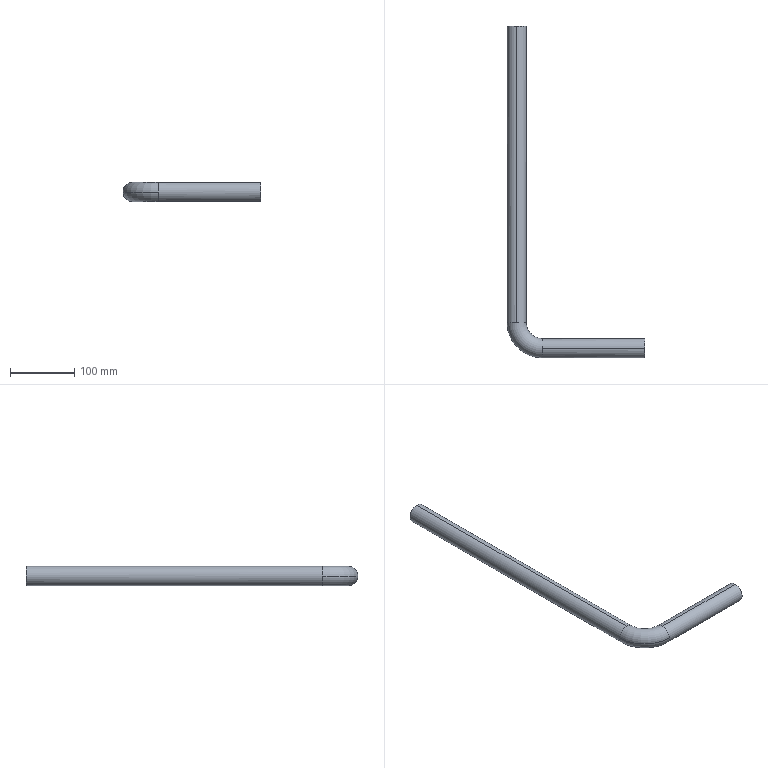Part | SolidWorks | features Sweep 1 | 1 solid | 14 faces | box 215 x 517 x 30 mm | volume 120482 mm3 | cylinder 8 | torus 4 | plane 2 | commonest cylinder face diameters 26 x4 30 x4
STEP:
#1=CARTESIAN_POINT('',(40.,0.,13.));
#2=VERTEX_POINT('',#1);
#3=CARTESIAN_POINT('',(40.,-13.,0.));
#4=VERTEX_POINT('',#3);
#5=CARTESIAN_POINT('',(40.,0.,0.));
#6=DIRECTION('',(1.,0.,0.));
#7=DIRECTION('',(0.,0.,1.));
#8=AXIS2_PLACEMENT_3D('',#5,#6,#7);
#9=CIRCLE('',#8,13.);
#10=EDGE_CURVE('',#2,#4,#9,.T.);
#11=ORIENTED_EDGE('',*,*,#10,.T.);
#12=CARTESIAN_POINT('',(-13.,40.,0.));
#13=VERTEX_POINT('',#12);
#14=CARTESIAN_POINT('',(40.,40.,0.));
#15=DIRECTION('',(0.,0.,-1.));
#16=DIRECTION('',(-1.,0.,0.));
#17=AXIS2_PLACEMENT_3D('',#14,#15,#16);
#18=CIRCLE('',#17,53.);
#19=EDGE_CURVE('',#4,#13,#18,.T.);
#20=ORIENTED_EDGE('',*,*,#19,.T.);
#21=CARTESIAN_POINT('',(0.,40.,13.));
#22=VERTEX_POINT('',#21);
#23=CARTESIAN_POINT('',(0.,40.,0.));
#24=DIRECTION('',(0.,-1.,0.));
#25=DIRECTION('',(0.,0.,-1.));
#26=AXIS2_PLACEMENT_3D('',#23,#24,#25);
#27=CIRCLE('',#26,13.);
#28=EDGE_CURVE('',#22,#13,#27,.T.);
#29=ORIENTED_EDGE('',*,*,#28,.F.);
#30=CARTESIAN_POINT('',(13.,40.,0.));
#31=VERTEX_POINT('',#30);
#32=CARTESIAN_POINT('',(0.,40.,0.));
#33=DIRECTION('',(0.,-1.,0.));
#34=DIRECTION('',(0.,0.,-1.));
#35=AXIS2_PLACEMENT_3D('',#32,#33,#34);
#36=CIRCLE('',#35,13.);
#37=EDGE_CURVE('',#31,#22,#36,.T.);
#38=ORIENTED_EDGE('',*,*,#37,.F.);
#39=CARTESIAN_POINT('',(40.,13.,0.));
#40=VERTEX_POINT('',#39);
#41=CARTESIAN_POINT('',(40.,40.,0.));
#42=DIRECTION('',(0.,0.,-1.));
#43=DIRECTION('',(-1.,0.,0.));
#44=AXIS2_PLACEMENT_3D('',#41,#42,#43);
#45=CIRCLE('',#44,27.);
#46=EDGE_CURVE('',#40,#31,#45,.T.);
#47=ORIENTED_EDGE('',*,*,#46,.F.);
#48=CARTESIAN_POINT('',(40.,0.,0.));
#49=DIRECTION('',(1.,0.,0.));
#50=DIRECTION('',(0.,0.,1.));
#51=AXIS2_PLACEMENT_3D('',#48,#49,#50);
#52=CIRCLE('',#51,13.);
#53=EDGE_CURVE('',#40,#2,#52,.T.);
#54=ORIENTED_EDGE('',*,*,#53,.T.);
#55=EDGE_LOOP('',(#11,#20,#29,#38,#47,#54));
#56=FACE_OUTER_BOUND('',#55,.T.);
#57=CARTESIAN_POINT('',(40.,40.,0.));
#58=DIRECTION('',(0.,0.,-1.));
#59=DIRECTION('',(-1.,0.,0.));
#60=AXIS2_PLACEMENT_3D('',#57,#58,#59);
#61=TOROIDAL_SURFACE('',#60,40.,13.);
#62=ADVANCED_FACE('',(#56),#61,.F.);
#63=CARTESIAN_POINT('',(40.,-15.,0.));
#64=VERTEX_POINT('',#63);
#65=CARTESIAN_POINT('',(40.,0.,-15.));
#66=VERTEX_POINT('',#65);
#67=CARTESIAN_POINT('',(40.,0.,0.));
#68=DIRECTION('',(1.,0.,0.));
#69=DIRECTION('',(0.,0.,-1.));
#70=AXIS2_PLACEMENT_3D('',#67,#68,#69);
#71=CIRCLE('',#70,15.);
#72=EDGE_CURVE('',#64,#66,#71,.T.);
#73=ORIENTED_EDGE('',*,*,#72,.F.);
#74=CARTESIAN_POINT('',(-15.,40.,0.));
#75=VERTEX_POINT('',#74);
#76=CARTESIAN_POINT('',(40.,40.,0.));
#77=DIRECTION('',(0.,0.,-1.));
#78=DIRECTION('',(-1.,0.,0.));
#79=AXIS2_PLACEMENT_3D('',#76,#77,#78);
#80=CIRCLE('',#79,55.);
#81=EDGE_CURVE('',#64,#75,#80,.T.);
#82=ORIENTED_EDGE('',*,*,#81,.T.);
#83=CARTESIAN_POINT('',(0.,40.,-15.));
#84=VERTEX_POINT('',#83);
#85=CARTESIAN_POINT('',(0.,40.,0.));
#86=DIRECTION('',(0.,-1.,0.));
#87=DIRECTION('',(0.,0.,-1.));
#88=AXIS2_PLACEMENT_3D('',#85,#86,#87);
#89=CIRCLE('',#88,15.);
#90=EDGE_CURVE('',#75,#84,#89,.T.);
#91=ORIENTED_EDGE('',*,*,#90,.T.);
#92=CARTESIAN_POINT('',(15.,40.,0.));
#93=VERTEX_POINT('',#92);
#94=CARTESIAN_POINT('',(0.,40.,0.));
#95=DIRECTION('',(0.,-1.,0.));
#96=DIRECTION('',(0.,0.,-1.));
#97=AXIS2_PLACEMENT_3D('',#94,#95,#96);
#98=CIRCLE('',#97,15.);
#99=EDGE_CURVE('',#84,#93,#98,.T.);
#100=ORIENTED_EDGE('',*,*,#99,.T.);
#101=CARTESIAN_POINT('',(40.,15.,0.));
#102=VERTEX_POINT('',#101);
#103=CARTESIAN_POINT('',(40.,40.,0.));
#104=DIRECTION('',(0.,0.,-1.));
#105=DIRECTION('',(-1.,0.,0.));
#106=AXIS2_PLACEMENT_3D('',#103,#104,#105);
#107=CIRCLE('',#106,25.);
#108=EDGE_CURVE('',#102,#93,#107,.T.);
#109=ORIENTED_EDGE('',*,*,#108,.F.);
#110=CARTESIAN_POINT('',(40.,0.,0.));
#111=DIRECTION('',(1.,0.,0.));
#112=DIRECTION('',(0.,0.,-1.));
#113=AXIS2_PLACEMENT_3D('',#110,#111,#112);
#114=CIRCLE('',#113,15.);
#115=EDGE_CURVE('',#66,#102,#114,.T.);
#116=ORIENTED_EDGE('',*,*,#115,.F.);
#117=EDGE_LOOP('',(#73,#82,#91,#100,#109,#116));
#118=FACE_OUTER_BOUND('',#117,.T.);
#119=CARTESIAN_POINT('',(40.,40.,0.));
#120=DIRECTION('',(0.,0.,-1.));
#121=DIRECTION('',(-1.,0.,0.));
#122=AXIS2_PLACEMENT_3D('',#119,#120,#121);
#123=TOROIDAL_SURFACE('',#122,40.,15.);
#124=ADVANCED_FACE('',(#118),#123,.T.);
#125=ORIENTED_EDGE('',*,*,#28,.T.);
#126=CARTESIAN_POINT('',(0.,40.,-13.));
#127=VERTEX_POINT('',#126);
#128=CARTESIAN_POINT('',(0.,40.,0.));
#129=DIRECTION('',(0.,-1.,0.));
#130=DIRECTION('',(0.,0.,-1.));
#131=AXIS2_PLACEMENT_3D('',#128,#129,#130);
#132=CIRCLE('',#131,13.);
#133=EDGE_CURVE('',#13,#127,#132,.T.);
#134=ORIENTED_EDGE('',*,*,#133,.T.);
#135=CARTESIAN_POINT('',(0.,502.,-13.));
#136=VERTEX_POINT('',#135);
#137=CARTESIAN_POINT('',(0.,40.,-13.));
#138=DIRECTION('',(0.,1.,0.));
#139=VECTOR('',#138,1000.);
#140=LINE('',#137,#139);
#141=EDGE_CURVE('',#127,#136,#140,.T.);
#142=ORIENTED_EDGE('',*,*,#141,.T.);
#143=CARTESIAN_POINT('',(0.,502.,13.));
#144=VERTEX_POINT('',#143);
#145=CARTESIAN_POINT('',(0.,502.,0.));
#146=DIRECTION('',(0.,-1.,0.));
#147=DIRECTION('',(0.,0.,-1.));
#148=AXIS2_PLACEMENT_3D('',#145,#146,#147);
#149=CIRCLE('',#148,13.);
#150=EDGE_CURVE('',#144,#136,#149,.T.);
#151=ORIENTED_EDGE('',*,*,#150,.F.);
#152=CARTESIAN_POINT('',(0.,40.,13.));
#153=DIRECTION('',(0.,1.,0.));
#154=VECTOR('',#153,1000.);
#155=LINE('',#152,#154);
#156=EDGE_CURVE('',#22,#144,#155,.T.);
#157=ORIENTED_EDGE('',*,*,#156,.F.);
#158=EDGE_LOOP('',(#125,#134,#142,#151,#157));
#159=FACE_OUTER_BOUND('',#158,.T.);
#160=CARTESIAN_POINT('',(0.,40.,0.));
#161=DIRECTION('',(0.,1.,0.));
#162=DIRECTION('',(0.,0.,1.));
#163=AXIS2_PLACEMENT_3D('',#160,#161,#162);
#164=CYLINDRICAL_SURFACE('',#163,13.);
#165=ADVANCED_FACE('',(#159),#164,.F.);
#166=CARTESIAN_POINT('',(200.,0.,13.));
#167=VERTEX_POINT('',#166);
#168=CARTESIAN_POINT('',(200.,0.,-13.));
#169=VERTEX_POINT('',#168);
#170=CARTESIAN_POINT('',(200.,0.,0.));
#171=DIRECTION('',(1.,0.,0.));
#172=DIRECTION('',(0.,0.,-1.));
#173=AXIS2_PLACEMENT_3D('',#170,#171,#172);
#174=CIRCLE('',#173,13.);
#175=EDGE_CURVE('',#167,#169,#174,.T.);
#176=ORIENTED_EDGE('',*,*,#175,.T.);
#177=CARTESIAN_POINT('',(40.,0.,-13.));
#178=VERTEX_POINT('',#177);
#179=CARTESIAN_POINT('',(200.,0.,-13.));
#180=DIRECTION('',(-1.,0.,0.));
#181=VECTOR('',#180,1000.);
#182=LINE('',#179,#181);
#183=EDGE_CURVE('',#169,#178,#182,.T.);
#184=ORIENTED_EDGE('',*,*,#183,.T.);
#185=CARTESIAN_POINT('',(40.,0.,0.));
#186=DIRECTION('',(1.,0.,0.));
#187=DIRECTION('',(0.,0.,1.));
#188=AXIS2_PLACEMENT_3D('',#185,#186,#187);
#189=CIRCLE('',#188,13.);
#190=EDGE_CURVE('',#4,#178,#189,.T.);
#191=ORIENTED_EDGE('',*,*,#190,.F.);
#192=ORIENTED_EDGE('',*,*,#10,.F.);
#193=CARTESIAN_POINT('',(200.,0.,13.));
#194=DIRECTION('',(-1.,0.,0.));
#195=VECTOR('',#194,1000.);
#196=LINE('',#193,#195);
#197=EDGE_CURVE('',#167,#2,#196,.T.);
#198=ORIENTED_EDGE('',*,*,#197,.F.);
#199=EDGE_LOOP('',(#176,#184,#191,#192,#198));
#200=FACE_OUTER_BOUND('',#199,.T.);
#201=CARTESIAN_POINT('',(200.,0.,0.));
#202=DIRECTION('',(-1.,0.,0.));
#203=DIRECTION('',(0.,0.,1.));
#204=AXIS2_PLACEMENT_3D('',#201,#202,#203);
#205=CYLINDRICAL_SURFACE('',#204,13.);
#206=ADVANCED_FACE('',(#200),#205,.F.);
#207=ORIENTED_EDGE('',*,*,#99,.F.);
#208=CARTESIAN_POINT('',(0.,502.,-15.));
#209=VERTEX_POINT('',#208);
#210=CARTESIAN_POINT('',(0.,40.,-15.));
#211=DIRECTION('',(0.,1.,0.));
#212=VECTOR('',#211,1000.);
#213=LINE('',#210,#212);
#214=EDGE_CURVE('',#84,#209,#213,.T.);
#215=ORIENTED_EDGE('',*,*,#214,.T.);
#216=CARTESIAN_POINT('',(0.,502.,15.));
#217=VERTEX_POINT('',#216);
#218=CARTESIAN_POINT('',(0.,502.,0.));
#219=DIRECTION('',(0.,-1.,0.));
#220=DIRECTION('',(0.,0.,-1.));
#221=AXIS2_PLACEMENT_3D('',#218,#219,#220);
#222=CIRCLE('',#221,15.);
#223=EDGE_CURVE('',#209,#217,#222,.T.);
#224=ORIENTED_EDGE('',*,*,#223,.T.);
#225=CARTESIAN_POINT('',(0.,40.,15.));
#226=VERTEX_POINT('',#225);
#227=CARTESIAN_POINT('',(0.,40.,15.));
#228=DIRECTION('',(0.,1.,0.));
#229=VECTOR('',#228,1000.);
#230=LINE('',#227,#229);
#231=EDGE_CURVE('',#226,#217,#230,.T.);
#232=ORIENTED_EDGE('',*,*,#231,.F.);
#233=CARTESIAN_POINT('',(0.,40.,0.));
#234=DIRECTION('',(0.,-1.,0.));
#235=DIRECTION('',(0.,0.,-1.));
#236=AXIS2_PLACEMENT_3D('',#233,#234,#235);
#237=CIRCLE('',#236,15.);
#238=EDGE_CURVE('',#93,#226,#237,.T.);
#239=ORIENTED_EDGE('',*,*,#238,.F.);
#240=EDGE_LOOP('',(#207,#215,#224,#232,#239));
#241=FACE_OUTER_BOUND('',#240,.T.);
#242=CARTESIAN_POINT('',(0.,40.,0.));
#243=DIRECTION('',(0.,1.,0.));
#244=DIRECTION('',(0.,0.,1.));
#245=AXIS2_PLACEMENT_3D('',#242,#243,#244);
#246=CYLINDRICAL_SURFACE('',#245,15.);
#247=ADVANCED_FACE('',(#241),#246,.T.);
#248=CARTESIAN_POINT('',(200.,0.,-15.));
#249=VERTEX_POINT('',#248);
#250=CARTESIAN_POINT('',(200.,0.,15.));
#251=VERTEX_POINT('',#250);
#252=CARTESIAN_POINT('',(200.,0.,0.));
#253=DIRECTION('',(1.,0.,0.));
#254=DIRECTION('',(0.,0.,-1.));
#255=AXIS2_PLACEMENT_3D('',#252,#253,#254);
#256=CIRCLE('',#255,15.);
#257=EDGE_CURVE('',#249,#251,#256,.T.);
#258=ORIENTED_EDGE('',*,*,#257,.F.);
#259=CARTESIAN_POINT('',(200.,0.,-15.));
#260=DIRECTION('',(-1.,0.,0.));
#261=VECTOR('',#260,1000.);
#262=LINE('',#259,#261);
#263=EDGE_CURVE('',#249,#66,#262,.T.);
#264=ORIENTED_EDGE('',*,*,#263,.T.);
#265=ORIENTED_EDGE('',*,*,#115,.T.);
#266=CARTESIAN_POINT('',(40.,0.,15.));
#267=VERTEX_POINT('',#266);
#268=CARTESIAN_POINT('',(40.,0.,0.));
#269=DIRECTION('',(1.,0.,0.));
#270=DIRECTION('',(0.,0.,-1.));
#271=AXIS2_PLACEMENT_3D('',#268,#269,#270);
#272=CIRCLE('',#271,15.);
#273=EDGE_CURVE('',#102,#267,#272,.T.);
#274=ORIENTED_EDGE('',*,*,#273,.T.);
#275=CARTESIAN_POINT('',(200.,0.,15.));
#276=DIRECTION('',(-1.,0.,0.));
#277=VECTOR('',#276,1000.);
#278=LINE('',#275,#277);
#279=EDGE_CURVE('',#251,#267,#278,.T.);
#280=ORIENTED_EDGE('',*,*,#279,.F.);
#281=EDGE_LOOP('',(#258,#264,#265,#274,#280));
#282=FACE_OUTER_BOUND('',#281,.T.);
#283=CARTESIAN_POINT('',(200.,0.,0.));
#284=DIRECTION('',(-1.,0.,0.));
#285=DIRECTION('',(0.,0.,1.));
#286=AXIS2_PLACEMENT_3D('',#283,#284,#285);
#287=CYLINDRICAL_SURFACE('',#286,15.);
#288=ADVANCED_FACE('',(#282),#287,.T.);
#289=ORIENTED_EDGE('',*,*,#214,.F.);
#290=ORIENTED_EDGE('',*,*,#90,.F.);
#291=CARTESIAN_POINT('',(0.,40.,0.));
#292=DIRECTION('',(0.,-1.,0.));
#293=DIRECTION('',(0.,0.,-1.));
#294=AXIS2_PLACEMENT_3D('',#291,#292,#293);
#295=CIRCLE('',#294,15.);
#296=EDGE_CURVE('',#226,#75,#295,.T.);
#297=ORIENTED_EDGE('',*,*,#296,.F.);
#298=ORIENTED_EDGE('',*,*,#231,.T.);
#299=CARTESIAN_POINT('',(0.,502.,0.));
#300=DIRECTION('',(0.,-1.,0.));
#301=DIRECTION('',(0.,0.,-1.));
#302=AXIS2_PLACEMENT_3D('',#299,#300,#301);
#303=CIRCLE('',#302,15.);
#304=EDGE_CURVE('',#217,#209,#303,.T.);
#305=ORIENTED_EDGE('',*,*,#304,.T.);
#306=EDGE_LOOP('',(#289,#290,#297,#298,#305));
#307=FACE_OUTER_BOUND('',#306,.T.);
#308=CARTESIAN_POINT('',(0.,40.,0.));
#309=DIRECTION('',(0.,1.,0.));
#310=DIRECTION('',(0.,0.,1.));
#311=AXIS2_PLACEMENT_3D('',#308,#309,#310);
#312=CYLINDRICAL_SURFACE('',#311,15.);
#313=ADVANCED_FACE('',(#307),#312,.T.);
#314=ORIENTED_EDGE('',*,*,#81,.F.);
#315=CARTESIAN_POINT('',(40.,0.,0.));
#316=DIRECTION('',(1.,0.,0.));
#317=DIRECTION('',(0.,0.,-1.));
#318=AXIS2_PLACEMENT_3D('',#315,#316,#317);
#319=CIRCLE('',#318,15.);
#320=EDGE_CURVE('',#267,#64,#319,.T.);
#321=ORIENTED_EDGE('',*,*,#320,.F.);
#322=ORIENTED_EDGE('',*,*,#273,.F.);
#323=ORIENTED_EDGE('',*,*,#108,.T.);
#324=ORIENTED_EDGE('',*,*,#238,.T.);
#325=ORIENTED_EDGE('',*,*,#296,.T.);
#326=EDGE_LOOP('',(#314,#321,#322,#323,#324,#325));
#327=FACE_OUTER_BOUND('',#326,.T.);
#328=CARTESIAN_POINT('',(40.,40.,0.));
#329=DIRECTION('',(0.,0.,-1.));
#330=DIRECTION('',(-1.,0.,0.));
#331=AXIS2_PLACEMENT_3D('',#328,#329,#330);
#332=TOROIDAL_SURFACE('',#331,40.,15.);
#333=ADVANCED_FACE('',(#327),#332,.T.);
#334=ORIENTED_EDGE('',*,*,#263,.F.);
#335=CARTESIAN_POINT('',(200.,0.,0.));
#336=DIRECTION('',(1.,0.,0.));
#337=DIRECTION('',(0.,0.,-1.));
#338=AXIS2_PLACEMENT_3D('',#335,#336,#337);
#339=CIRCLE('',#338,15.);
#340=EDGE_CURVE('',#251,#249,#339,.T.);
#341=ORIENTED_EDGE('',*,*,#340,.F.);
#342=ORIENTED_EDGE('',*,*,#279,.T.);
#343=ORIENTED_EDGE('',*,*,#320,.T.);
#344=ORIENTED_EDGE('',*,*,#72,.T.);
#345=EDGE_LOOP('',(#334,#341,#342,#343,#344));
#346=FACE_OUTER_BOUND('',#345,.T.);
#347=CARTESIAN_POINT('',(200.,0.,0.));
#348=DIRECTION('',(-1.,0.,0.));
#349=DIRECTION('',(0.,0.,1.));
#350=AXIS2_PLACEMENT_3D('',#347,#348,#349);
#351=CYLINDRICAL_SURFACE('',#350,15.);
#352=ADVANCED_FACE('',(#346),#351,.T.);
#353=ORIENTED_EDGE('',*,*,#150,.T.);
#354=CARTESIAN_POINT('',(0.,502.,0.));
#355=DIRECTION('',(0.,-1.,0.));
#356=DIRECTION('',(0.,0.,-1.));
#357=AXIS2_PLACEMENT_3D('',#354,#355,#356);
#358=CIRCLE('',#357,13.);
#359=EDGE_CURVE('',#136,#144,#358,.T.);
#360=ORIENTED_EDGE('',*,*,#359,.T.);
#361=EDGE_LOOP('',(#353,#360));
#362=FACE_BOUND('',#361,.T.);
#363=ORIENTED_EDGE('',*,*,#304,.F.);
#364=ORIENTED_EDGE('',*,*,#223,.F.);
#365=EDGE_LOOP('',(#363,#364));
#366=FACE_OUTER_BOUND('',#365,.T.);
#367=CARTESIAN_POINT('',(0.,502.,0.));
#368=DIRECTION('',(0.,-1.,0.));
#369=DIRECTION('',(0.,0.,-1.));
#370=AXIS2_PLACEMENT_3D('',#367,#368,#369);
#371=PLANE('',#370);
#372=ADVANCED_FACE('',(#362,#366),#371,.F.);
#373=ORIENTED_EDGE('',*,*,#175,.F.);
#374=CARTESIAN_POINT('',(200.,0.,0.));
#375=DIRECTION('',(1.,0.,0.));
#376=DIRECTION('',(0.,0.,-1.));
#377=AXIS2_PLACEMENT_3D('',#374,#375,#376);
#378=CIRCLE('',#377,13.);
#379=EDGE_CURVE('',#169,#167,#378,.T.);
#380=ORIENTED_EDGE('',*,*,#379,.F.);
#381=EDGE_LOOP('',(#373,#380));
#382=FACE_BOUND('',#381,.T.);
#383=ORIENTED_EDGE('',*,*,#340,.T.);
#384=ORIENTED_EDGE('',*,*,#257,.T.);
#385=EDGE_LOOP('',(#383,#384));
#386=FACE_OUTER_BOUND('',#385,.T.);
#387=CARTESIAN_POINT('',(200.,0.,0.));
#388=DIRECTION('',(1.,0.,0.));
#389=DIRECTION('',(0.,0.,-1.));
#390=AXIS2_PLACEMENT_3D('',#387,#388,#389);
#391=PLANE('',#390);
#392=ADVANCED_FACE('',(#382,#386),#391,.T.);
#393=ORIENTED_EDGE('',*,*,#141,.F.);
#394=CARTESIAN_POINT('',(0.,40.,0.));
#395=DIRECTION('',(0.,-1.,0.));
#396=DIRECTION('',(0.,0.,-1.));
#397=AXIS2_PLACEMENT_3D('',#394,#395,#396);
#398=CIRCLE('',#397,13.);
#399=EDGE_CURVE('',#127,#31,#398,.T.);
#400=ORIENTED_EDGE('',*,*,#399,.T.);
#401=ORIENTED_EDGE('',*,*,#37,.T.);
#402=ORIENTED_EDGE('',*,*,#156,.T.);
#403=ORIENTED_EDGE('',*,*,#359,.F.);
#404=EDGE_LOOP('',(#393,#400,#401,#402,#403));
#405=FACE_OUTER_BOUND('',#404,.T.);
#406=CARTESIAN_POINT('',(0.,40.,0.));
#407=DIRECTION('',(0.,1.,0.));
#408=DIRECTION('',(0.,0.,1.));
#409=AXIS2_PLACEMENT_3D('',#406,#407,#408);
#410=CYLINDRICAL_SURFACE('',#409,13.);
#411=ADVANCED_FACE('',(#405),#410,.F.);
#412=ORIENTED_EDGE('',*,*,#19,.F.);
#413=ORIENTED_EDGE('',*,*,#190,.T.);
#414=CARTESIAN_POINT('',(40.,0.,0.));
#415=DIRECTION('',(1.,0.,0.));
#416=DIRECTION('',(0.,0.,1.));
#417=AXIS2_PLACEMENT_3D('',#414,#415,#416);
#418=CIRCLE('',#417,13.);
#419=EDGE_CURVE('',#178,#40,#418,.T.);
#420=ORIENTED_EDGE('',*,*,#419,.T.);
#421=ORIENTED_EDGE('',*,*,#46,.T.);
#422=ORIENTED_EDGE('',*,*,#399,.F.);
#423=ORIENTED_EDGE('',*,*,#133,.F.);
#424=EDGE_LOOP('',(#412,#413,#420,#421,#422,#423));
#425=FACE_OUTER_BOUND('',#424,.T.);
#426=CARTESIAN_POINT('',(40.,40.,0.));
#427=DIRECTION('',(0.,0.,-1.));
#428=DIRECTION('',(-1.,0.,0.));
#429=AXIS2_PLACEMENT_3D('',#426,#427,#428);
#430=TOROIDAL_SURFACE('',#429,40.,13.);
#431=ADVANCED_FACE('',(#425),#430,.F.);
#432=ORIENTED_EDGE('',*,*,#183,.F.);
#433=ORIENTED_EDGE('',*,*,#379,.T.);
#434=ORIENTED_EDGE('',*,*,#197,.T.);
#435=ORIENTED_EDGE('',*,*,#53,.F.);
#436=ORIENTED_EDGE('',*,*,#419,.F.);
#437=EDGE_LOOP('',(#432,#433,#434,#435,#436));
#438=FACE_OUTER_BOUND('',#437,.T.);
#439=CARTESIAN_POINT('',(200.,0.,0.));
#440=DIRECTION('',(-1.,0.,0.));
#441=DIRECTION('',(0.,0.,1.));
#442=AXIS2_PLACEMENT_3D('',#439,#440,#441);
#443=CYLINDRICAL_SURFACE('',#442,13.);
#444=ADVANCED_FACE('',(#438),#443,.F.);
#445=CLOSED_SHELL('',(#62,#124,#165,#206,#247,#288,#313,#333,#352,#372,#392,#411,#431,#444));
#446=MANIFOLD_SOLID_BREP('',#445);
#447=CARTESIAN_POINT('',(0.,0.,0.));
#448=DIRECTION('',(0.,0.,1.));
#449=DIRECTION('',(1.,0.,0.));
#450=AXIS2_PLACEMENT_3D('',#447,#448,#449);
#451=(LENGTH_UNIT()NAMED_UNIT(*)SI_UNIT(.MILLI.,.METRE.));
#452=UNCERTAINTY_MEASURE_WITH_UNIT(LENGTH_MEASURE(0.00001),#451,'','');
#453=(NAMED_UNIT(*)PLANE_ANGLE_UNIT()SI_UNIT($,.RADIAN.));
#454=(NAMED_UNIT(*)SI_UNIT($,.STERADIAN.)SOLID_ANGLE_UNIT());
#455=(GEOMETRIC_REPRESENTATION_CONTEXT(3)GLOBAL_UNCERTAINTY_ASSIGNED_CONTEXT((#452))GLOBAL_UNIT_ASSIGNED_CONTEXT((#451,#453,#454))REPRESENTATION_CONTEXT('',''));
#456=ADVANCED_BREP_SHAPE_REPRESENTATION('',(#446,#450),#455);